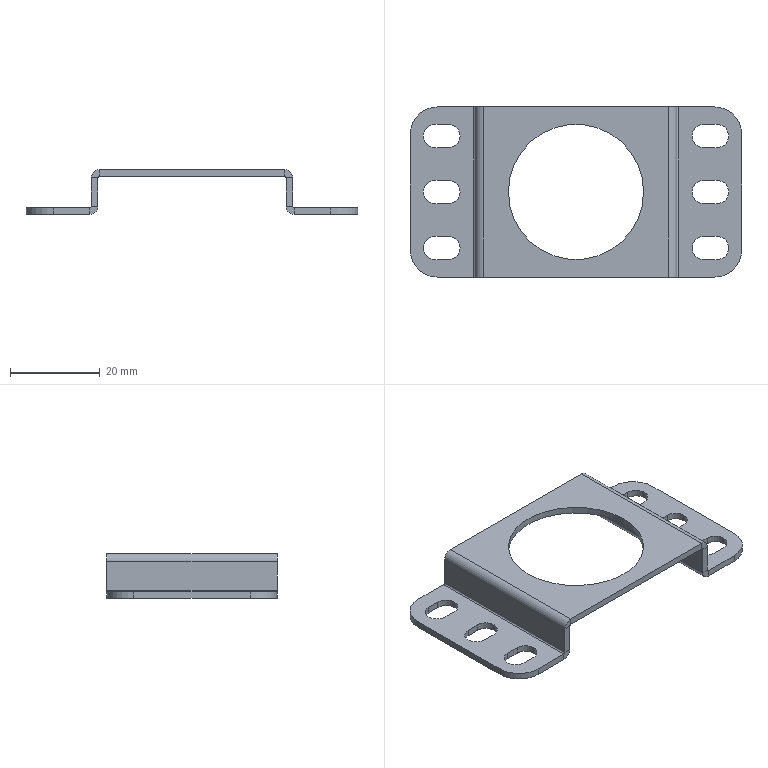Part | SolidWorks | features EdgeFlange 2, Fillet 1, FlatPattern 1, HoleWzd 1, ICE 1, SMBaseFlange 1, SheetMetal 1 | 1 solid | 74 faces | box 74 x 38 x 10 mm | volume 3632 mm3 | plane 42 | cylinder 32 | commonest cylinder face diameters 5.2 x18 0.6 x4 3.6 x4 12 x4 30.2 x2